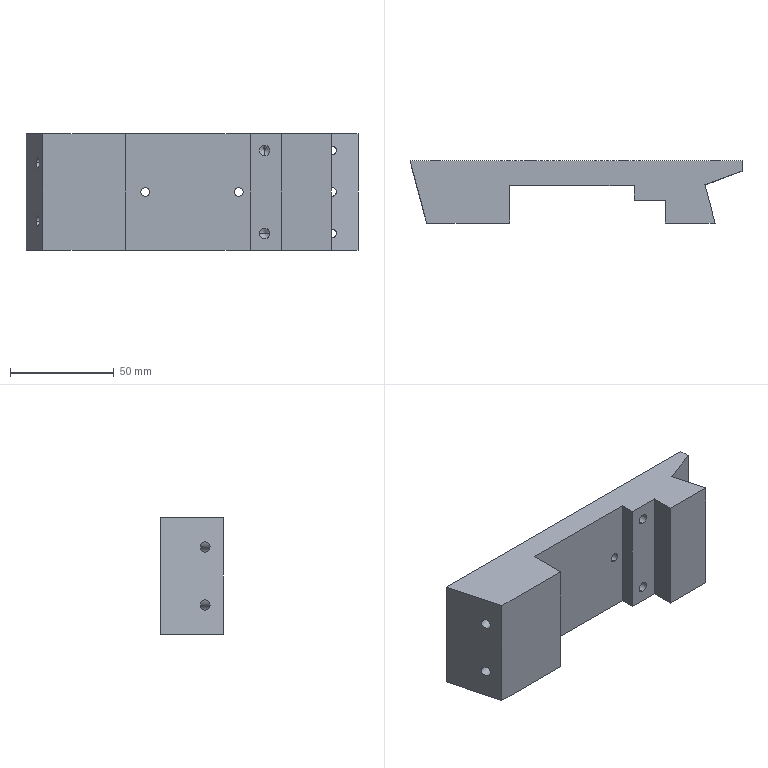Part | SolidWorks | features BaseBody 1 | 1 solid | 60 faces | box 160 x 30 x 56 mm | volume 169757 mm3 | cylinder 28 | cone 18 | plane 14 | commonest cylinder face diameters 4.2 x16 5 x12